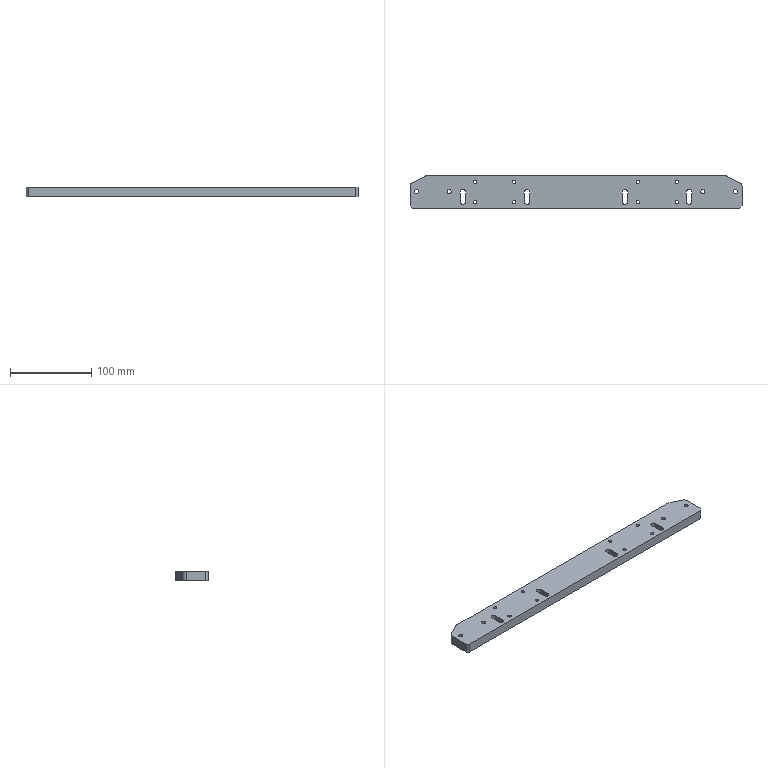CAM job | NX | 3-axis milling, drilling | part box 408 x 40 x 12 mm | stock box 413 x 45 x 15 mm
Tools:
number,name,description,diameter,corner_radius,flute_length,length,flutes
4,D4,平底铣刀-粗,4.0,0.0,25.0,75.0,2
6,D6,平底铣刀-粗,6.0,0.0,25.0,75.0,2
9,D10,平底铣刀-粗,10.0,0.0,35.0,75.0,2
11,D4-J,平底铣刀-精,4.0,0.0,50.0,75.0,2
7,D6-J,平底铣刀-精,6.0,0.0,25.0,75.0,2
10,D10-J,平底铣刀-精,10.0,0.0,35.0,75.0,2
1,D80R0.8飞刀,圆鼻刀-粗,80.0,0.8,50.0,75.0,2
1,D80R0.8飞刀-J,圆鼻刀-精,80.0,0.8,50.0,75.0,2
2,D6倒角刀,倒角刀,6.0,0.0,3.0,25.0,2
22,M5X0.8,丝锥,4.2,0.0,35.0,50.0,2
19,M6X1.0,丝锥,5.0,0.0,35.0,50.0,2
15,ZT5,钻头,5.0,0.0,35.0,50.0,2
14,钻头4.2,Twist Drill 4.2 mm,4.2,0.0,41.0,41.738,2
Operations:
program,operation,operation_type,tool,method,geometry_group,spindle_rpm,surface_speed,feed_per_tooth,feed_cut,feed_plunge,cut_length_mm,path_length_mm,cut_time_min,machine_time_min
B,FLOORWALLFACEROUGH_COPY,VolumeBased25DMillingOperation,D80R0.8飞刀,LAYERROUGH-DEPTHK-STEPG,W-B,2800.0,703.696,0.5357,3000.0,100.0,2580.97,4698.947,0.8603,1.072
B,FLOORWALLFACEFINISH_COPY,VolumeBased25DMillingOperation,D80R0.8飞刀-J,SIDEFINISH-DEPTHK-STEPG,W-B,4000.0,1005.28,0.125,1000.0,100.0,515.998,551.998,0.516,0.5196
B,DRILLCHAMFER_1,Operation,D6倒角刀,METHOD,W-B,8000.0,150.796,0.0625,1000.0,0.0,45.6,501.134,0.0456,0.0912
B,MILLCHAMFER_3,PlanarMilling,D6倒角刀,METHOD,W-B,8000.0,150.796,0.0375,600.0,100.0,75.821,635.101,0.1264,0.1823
B,PLANARDEBURR6X45L_COPY,SurfaceContour,D6倒角刀,SURFACECHAMFER-DEPTH0-STEPG,W-B,6500.0,122.519,0.1154,1500.0,100.0,1194.247,2243.141,0.7962,0.9011
A,TOPFACE,FaceMilling,D80R0.8飞刀,SIDEFINISH-DEPTHK-STEPG,W-A,4000.0,1005.31,0.125,1000.0,100.0,502.0,538.0,0.502,0.5056
A,PROFILEROUGH_2,VolumeBased25DMillingOperation,D10,METHOD,W-A,8000.0,251.327,0.3125,5000.0,80.0,15435.411,15486.111,3.087,3.092
A,SPOTDRILL-DEPTH0.8,Operation,D6倒角刀,NONE,W-A,8000.0,150.796,0.0312,500.0,90.0,21.6,591.438,0.0432,0.1002
A,THROUGHHOLE-M5TAPDRILL,Operation,钻头4.2,NONE,W-A,3000.0,39.584,0.0583,350.0,90.0,162.095,719.293,0.4631,0.5188
A,THROUGHHOLE-M6TAPDRILL,Operation,ZT5,NONE,W-A,2800.0,43.982,0.0625,350.0,90.0,82.009,599.044,0.2343,0.286
A,BLINDSLOTROUGH,VolumeBased25DMillingOperation,D6,METHOD,W-A,6000.0,113.097,0.1667,2000.0,100.0,3914.066,4366.873,1.957,2.002
A,THROUGHSLOTROUGH_1,VolumeBased25DMillingOperation,D4,METHOD,W-A,6000.0,75.398,0.1,1200.0,100.0,3412.398,3918.802,2.844,2.894
A,SLOTFINISH,VolumeBased25DMillingOperation,D6-J,METHOD,W-A,6000.0,113.0,0.0667,600.0,100.0,167.745,648.455,0.2796,0.3276
A,SLOTFINISH_3,VolumeBased25DMillingOperation,D4-J,METHOD,W-A,6000.0,113.0,0.0417,500.0,100.0,275.172,835.482,0.5503,0.6064
A,BODYONLY,SurfaceContour,D6倒角刀,METHOD,W-A,8000.0,150.796,0.1875,3000.0,100.0,1131.285,1718.41,0.3771,0.4358
A,MILLCHAMFER_1,PlanarMilling,D6倒角刀,METHOD,W-A,8000.0,150.796,0.0312,500.0,100.0,144.163,820.209,0.2883,0.3559
A,MILLCHAMFER_2,PlanarMilling,D6倒角刀,METHOD,W-A,8000.0,150.796,0.0312,500.0,100.0,79.753,636.664,0.1595,0.2152
A,THROUGHHOLE-TAPM5,Operation,M5X0.8,METHOD,W-A,500.0,6.597,0.0008,0.8,90.0,132.0,659.104,165.0,165.053
A,THROUGHHOLE-TAPM6,Operation,M6X1.0,METHOD,W-A,500.0,7.854,0.001,1.0,90.0,66.0,567.027,66.0,66.05
A,PROFILESEMIFINISH_2,VolumeBased25DMillingOperation,D10-J,METHOD,W-A,8000.0,251.327,0.0625,1000.0,100.0,912.207,975.607,0.9122,0.9185